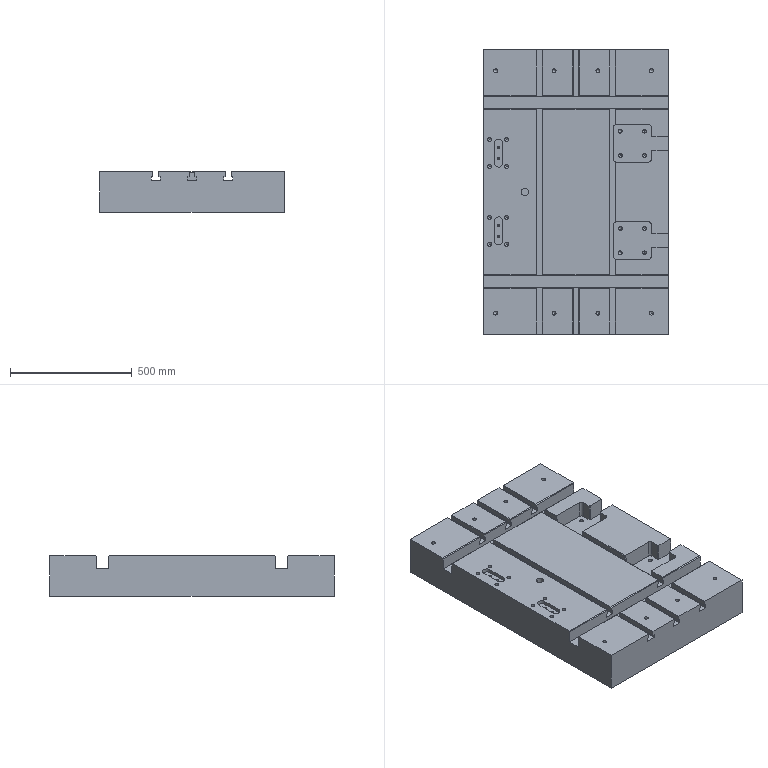Part | 1 solid | 329 faces | box 760 x 1170 x 165 mm | volume 135975153 mm3 | plane 161 | cylinder 74 | cone 72 | other 22 | commonest cylinder face diameters 16 x32 14 x16 20 x12 10 x8 35.02 x4 30 x2